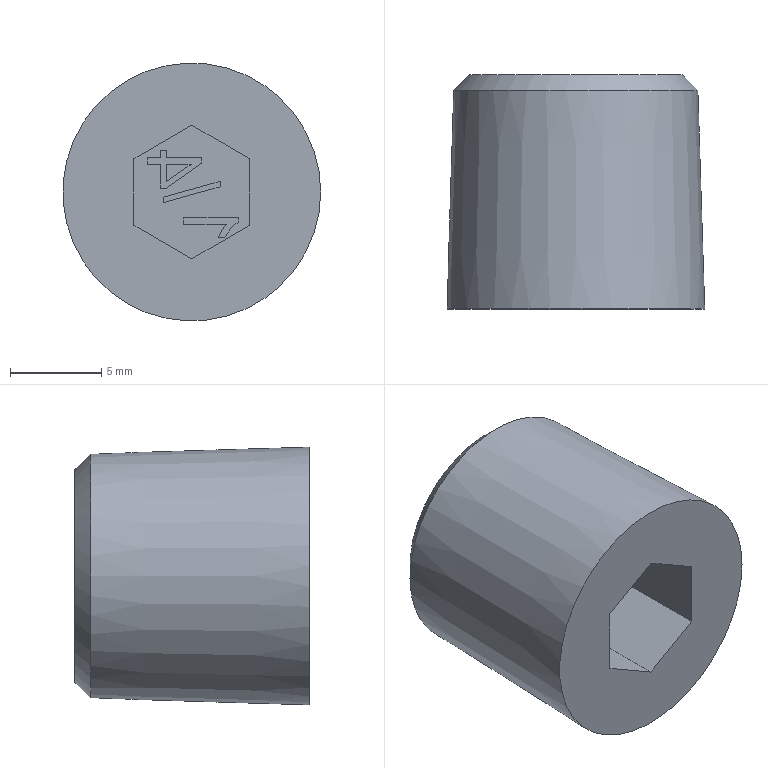Part | STEP file | solid 24 | 1 solid | 40 faces | box 14.157 x 12.856 x 14.157 mm | volume 1616 mm3 | plane 36 | cone 2 | other 2